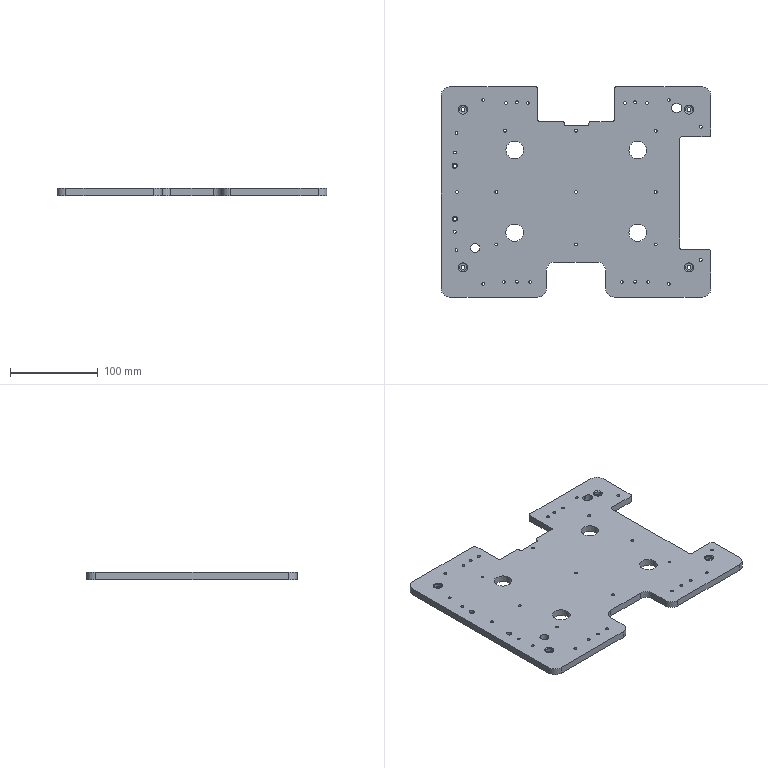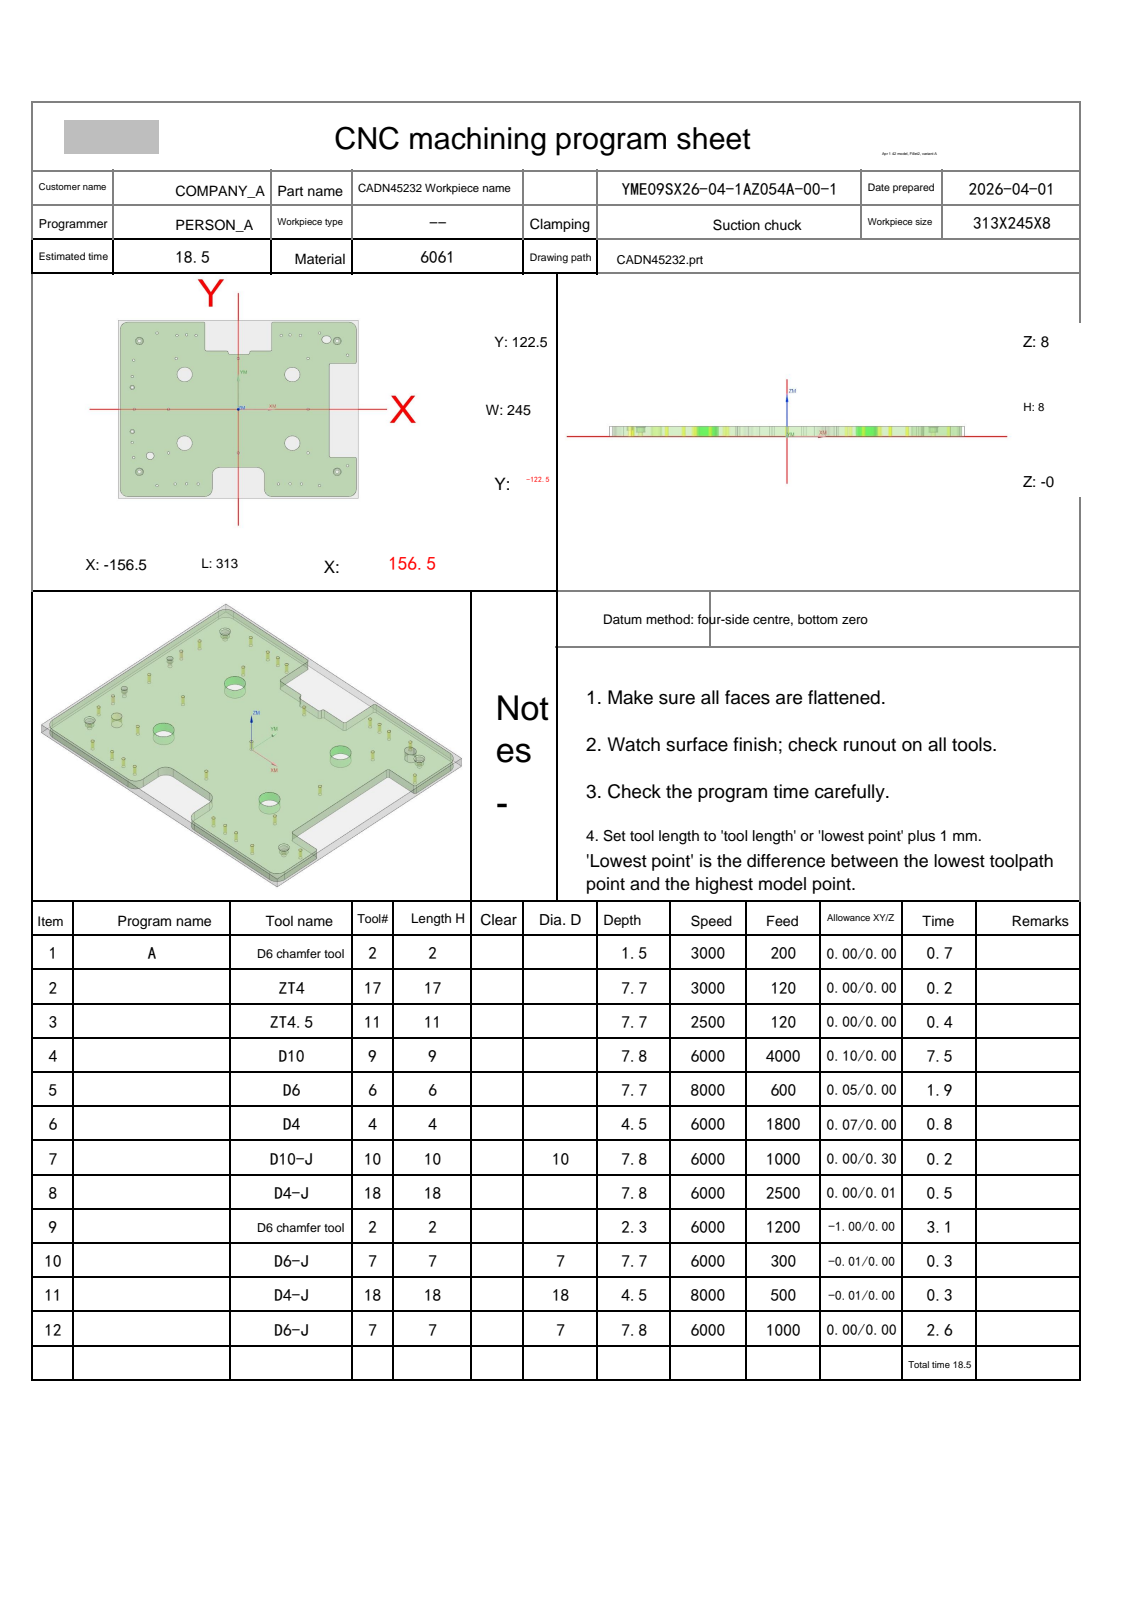NC program | NX | posted by the shop | part box 308 x 240 x 8 mm
Lines 1899 to 2964 of 6786:
N8 T18 M06
(D4-J  D=4. R=0. H=18 ce=0.00 di=0.01)
G00 G90 G54 X-40.899 Y85.842 M03 S6000
G43 H18 Z28.
M08
Z8.3
G01 X-40.906 Y85.841 Z8.214 F2000.
X-40.925 Y85.838 Z8.136
X-40.955 Y85.832 Z8.066
X-40.993 Y85.824 Z8.004
X-41.039 Y85.814 Z7.948
X-41.089 Y85.8 Z7.899
X-41.144 Y85.783 Z7.857
X-41.2 Y85.762 Z7.82
X-41.256 Y85.737 Z7.789
X-41.31 Y85.709 Z7.763
X-41.361 Y85.676 Z7.742
X-41.406 Y85.639 Z7.726
X-41.445 Y85.598 Z7.714
X-41.474 Y85.551 Z7.706
X-41.493 Y85.499 Z7.701
X-41.5 Y85.442 Z7.7
Y82.291 F2500.
X-41.459 Y82.289
X-41.387 Y82.303 Z7.699
X-41.308 Y82.349 Z7.695
X-41.224 Y82.423 Z7.689
X-41.138 Y82.521 Z7.681
X-41.053 Y82.641 Z7.671
X-40.972 Y82.779 Z7.659
X-40.897 Y82.932 Z7.647
X-40.832 Y83.096 Z7.633
X-40.78 Y83.268 Z7.619
X-40.729 Y83.535 Z7.596
X-40.711 Y83.806 Z7.573
X-40.724 Y84.078 Z7.55
X-40.767 Y84.344 Z7.527
X-40.836 Y84.6 Z7.504
X-40.931 Y84.84 Z7.481
X-40.999 Y84.975 Z7.468
X-41.072 Y85.1 Z7.456
X-41.148 Y85.212 Z7.444
X-41.224 Y85.309 Z7.434
X-41.296 Y85.39 Z7.424
X-41.361 Y85.45 Z7.416
X-41.418 Y85.488 Z7.409
X-41.461 Y85.5 Z7.404
X-41.49 Y85.486 Z7.401
X-41.5 Y85.442 Z7.4
Y82.291
X-41.459 Y82.289
X-41.387 Y82.303 Z7.399
X-41.308 Y82.349 Z7.395
X-41.224 Y82.422 Z7.39
X-41.138 Y82.521 Z7.382
X-41.053 Y82.641 Z7.373
X-40.972 Y82.779 Z7.363
X-40.897 Y82.931 Z7.351
X-40.832 Y83.095 Z7.338
X-40.78 Y83.267 Z7.324
X-40.729 Y83.534 Z7.302
X-40.711 Y83.805 Z7.279
X-40.724 Y84.077 Z7.255
X-40.767 Y84.343 Z7.231
X-40.836 Y84.599 Z7.207
X-40.931 Y84.84 Z7.184
X-40.999 Y84.975 Z7.171
X-41.072 Y85.099 Z7.158
X-41.148 Y85.212 Z7.146
X-41.224 Y85.309 Z7.135
X-41.296 Y85.389 Z7.125
X-41.361 Y85.45 Z7.117
X-41.418 Y85.487 Z7.11
X-41.461 Y85.5 Z7.104
X-41.49 Y85.486 Z7.101
X-41.5 Y85.442 Z7.1
Y82.291
X-41.459 Y82.289
X-41.387 Y82.303 Z7.099
X-41.308 Y82.349 Z7.095
X-41.224 Y82.422 Z7.09
X-41.138 Y82.521 Z7.082
X-41.053 Y82.64 Z7.073
X-40.971 Y82.778 Z7.063
X-40.897 Y82.931 Z7.051
X-40.832 Y83.094 Z7.038
X-40.78 Y83.266 Z7.024
X-40.729 Y83.532 Z7.002
X-40.711 Y83.804 Z6.979
X-40.724 Y84.076 Z6.955
X-40.766 Y84.342 Z6.931
X-40.836 Y84.598 Z6.907
X-40.931 Y84.839 Z6.884
X-40.999 Y84.974 Z6.871
X-41.072 Y85.099 Z6.858
X-41.148 Y85.211 Z6.846
X-41.224 Y85.309 Z6.835
X-41.296 Y85.389 Z6.825
X-41.361 Y85.449 Z6.817
X-41.418 Y85.487 Z6.81
X-41.461 Y85.5 Z6.804
X-41.49 Y85.486 Z6.801
X-41.5 Y85.442 Z6.8
Y82.291
X-41.459 Y82.289
X-41.387 Y82.303 Z6.799
X-41.308 Y82.348 Z6.795
X-41.224 Y82.422 Z6.79
X-41.138 Y82.52 Z6.782
X-41.053 Y82.64 Z6.773
X-40.971 Y82.777 Z6.762
X-40.897 Y82.93 Z6.75
X-40.832 Y83.093 Z6.737
X-40.779 Y83.265 Z6.724
X-40.729 Y83.531 Z6.702
X-40.711 Y83.803 Z6.678
X-40.724 Y84.075 Z6.655
X-40.766 Y84.341 Z6.631
X-40.836 Y84.598 Z6.607
X-40.931 Y84.839 Z6.584
X-40.999 Y84.974 Z6.571
X-41.072 Y85.098 Z6.558
X-41.148 Y85.211 Z6.546
X-41.224 Y85.309 Z6.535
X-41.296 Y85.389 Z6.525
X-41.361 Y85.449 Z6.517
X-41.418 Y85.487 Z6.51
X-41.461 Y85.5 Z6.504
X-41.49 Y85.486 Z6.501
X-41.5 Y85.442 Z6.5
Y82.291
X-41.459 Y82.289
X-41.387 Y82.303 Z6.499
X-41.308 Y82.348 Z6.495
X-41.224 Y82.422 Z6.49
X-41.138 Y82.52 Z6.482
X-41.053 Y82.639 Z6.473
X-40.971 Y82.777 Z6.462
X-40.897 Y82.929 Z6.45
X-40.832 Y83.092 Z6.437
X-40.779 Y83.264 Z6.423
X-40.729 Y83.53 Z6.401
X-40.711 Y83.802 Z6.378
X-40.724 Y84.074 Z6.355
X-40.766 Y84.34 Z6.331
X-40.836 Y84.597 Z6.307
X-40.931 Y84.838 Z6.284
X-40.999 Y84.973 Z6.271
X-41.072 Y85.098 Z6.258
X-41.148 Y85.211 Z6.246
X-41.224 Y85.308 Z6.235
X-41.296 Y85.389 Z6.225
X-41.361 Y85.449 Z6.217
X-41.418 Y85.487 Z6.21
X-41.461 Y85.5 Z6.204
X-41.49 Y85.486 Z6.201
X-41.5 Y85.442 Z6.2
Y82.291
X-41.459 Y82.289
X-41.387 Y82.303 Z6.199
X-41.308 Y82.348 Z6.195
X-41.224 Y82.421 Z6.19
X-41.138 Y82.519 Z6.182
X-41.053 Y82.639 Z6.173
X-40.971 Y82.776 Z6.162
X-40.897 Y82.928 Z6.15
X-40.832 Y83.092 Z6.137
X-40.779 Y83.263 Z6.123
X-40.729 Y83.529 Z6.101
X-40.711 Y83.801 Z6.078
X-40.724 Y84.073 Z6.054
X-40.766 Y84.339 Z6.03
X-40.836 Y84.596 Z6.007
X-40.931 Y84.837 Z5.984
X-40.999 Y84.973 Z5.97
X-41.072 Y85.098 Z5.958
X-41.148 Y85.21 Z5.946
X-41.224 Y85.308 Z5.935
X-41.296 Y85.389 Z5.925
X-41.361 Y85.449 Z5.916
X-41.418 Y85.487 Z5.91
X-41.461 Y85.5 Z5.904
X-41.49 Y85.486 Z5.901
X-41.5 Y85.442 Z5.9
Y82.291
X-41.459 Y82.289
X-41.387 Y82.303 Z5.899
X-41.308 Y82.348 Z5.895
X-41.224 Y82.421 Z5.89
X-41.138 Y82.519 Z5.882
X-41.053 Y82.638 Z5.873
X-40.971 Y82.775 Z5.862
X-40.897 Y82.927 Z5.85
X-40.832 Y83.091 Z5.837
X-40.779 Y83.262 Z5.823
X-40.728 Y83.528 Z5.801
X-40.711 Y83.8 Z5.778
X-40.724 Y84.071 Z5.754
X-40.766 Y84.338 Z5.73
X-40.836 Y84.595 Z5.707
X-40.931 Y84.837 Z5.684
X-40.999 Y84.972 Z5.67
X-41.072 Y85.097 Z5.658
X-41.148 Y85.21 Z5.646
X-41.224 Y85.308 Z5.635
X-41.296 Y85.388 Z5.625
X-41.361 Y85.449 Z5.616
X-41.418 Y85.487 Z5.61
X-41.461 Y85.5 Z5.604
X-41.49 Y85.486 Z5.601
X-41.5 Y85.442 Z5.6
Y82.291
X-41.422 Y82.289
X-41.351 Y82.304 Z5.599
X-41.272 Y82.351 Z5.595
X-41.188 Y82.426 Z5.59
X-41.103 Y82.525 Z5.582
X-41.019 Y82.646 Z5.573
X-40.94 Y82.784 Z5.562
X-40.867 Y82.937 Z5.55
X-40.803 Y83.101 Z5.537
X-40.753 Y83.273 Z5.523
X-40.705 Y83.54 Z5.501
X-40.69 Y83.811 Z5.478
X-40.706 Y84.082 Z5.455
X-40.751 Y84.347 Z5.431
X-40.823 Y84.603 Z5.407
X-40.921 Y84.843 Z5.384
X-40.991 Y84.977 Z5.371
X-41.065 Y85.101 Z5.358
X-41.143 Y85.213 Z5.346
X-41.22 Y85.31 Z5.335
X-41.293 Y85.39 Z5.325
X-41.359 Y85.45 Z5.317
X-41.416 Y85.488 Z5.31
X-41.461 Y85.501 Z5.304
X-41.49 Y85.486 Z5.301
X-41.5 Y85.442 Z5.3
Y82.291
X-41.422 Y82.289
X-41.351 Y82.304 Z5.299
X-41.272 Y82.351 Z5.295
X-41.188 Y82.425 Z5.29
X-41.103 Y82.524 Z5.282
X-41.019 Y82.645 Z5.273
X-40.939 Y82.783 Z5.262
X-40.866 Y82.936 Z5.25
X-40.803 Y83.1 Z5.237
X-40.753 Y83.272 Z5.223
X-40.705 Y83.538 Z5.201
X-40.69 Y83.809 Z5.178
X-40.706 Y84.08 Z5.154
X-40.751 Y84.346 Z5.13
X-40.823 Y84.602 Z5.107
X-40.921 Y84.842 Z5.084
X-40.99 Y84.976 Z5.07
X-41.065 Y85.101 Z5.058
X-41.143 Y85.213 Z5.046
X-41.22 Y85.31 Z5.035
X-41.293 Y85.39 Z5.025
X-41.359 Y85.45 Z5.016
X-41.416 Y85.488 Z5.01
X-41.461 Y85.501 Z5.004
X-41.49 Y85.486 Z5.001
X-41.5 Y85.442 Z5.
Y82.291
X-41.422 Y82.289
X-41.351 Y82.304 Z4.999
X-41.272 Y82.351 Z4.995
X-41.188 Y82.425 Z4.99
X-41.103 Y82.524 Z4.982
X-41.019 Y82.644 Z4.973
X-40.939 Y82.782 Z4.962
X-40.866 Y82.935 Z4.95
X-40.803 Y83.099 Z4.937
X-40.752 Y83.27 Z4.923
X-40.704 Y83.536 Z4.901
X-40.689 Y83.808 Z4.878
X-40.706 Y84.079 Z4.854
X-40.751 Y84.345 Z4.83
X-40.823 Y84.601 Z4.807
X-40.921 Y84.841 Z4.784
X-40.99 Y84.976 Z4.77
X-41.065 Y85.1 Z4.758
X-41.143 Y85.212 Z4.746
X-41.22 Y85.31 Z4.735
X-41.293 Y85.39 Z4.725
X-41.359 Y85.45 Z4.716
X-41.416 Y85.488 Z4.71
X-41.461 Y85.501 Z4.704
X-41.49 Y85.486 Z4.701
X-41.5 Y85.442 Z4.7
Y82.291
X-41.422 Y82.289
X-41.351 Y82.304 Z4.699
X-41.272 Y82.351 Z4.695
X-41.188 Y82.426 Z4.689
X-41.103 Y82.525 Z4.681
X-41.019 Y82.646 Z4.671
X-40.94 Y82.784 Z4.659
X-40.866 Y82.937 Z4.647
X-40.803 Y83.101 Z4.633
X-40.753 Y83.273 Z4.619
X-40.705 Y83.54 Z4.596
X-40.69 Y83.811 Z4.573
X-40.706 Y84.082 Z4.55
X-40.751 Y84.347 Z4.527
X-40.823 Y84.603 Z4.504
X-40.921 Y84.843 Z4.481
X-40.991 Y84.977 Z4.468
X-41.065 Y85.101 Z4.456
X-41.143 Y85.213 Z4.444
X-41.22 Y85.31 Z4.434
X-41.293 Y85.39 Z4.424
X-41.359 Y85.45 Z4.416
X-41.416 Y85.488 Z4.409
X-41.461 Y85.501 Z4.404
X-41.49 Y85.486 Z4.401
X-41.5 Y85.442 Z4.4
Y82.291
X-41.422 Y82.289
X-41.351 Y82.304 Z4.399
X-41.272 Y82.351 Z4.395
X-41.188 Y82.425 Z4.389
X-41.103 Y82.524 Z4.381
X-41.019 Y82.645 Z4.371
X-40.939 Y82.783 Z4.359
X-40.866 Y82.936 Z4.347
X-40.803 Y83.1 Z4.333
X-40.752 Y83.272 Z4.319
X-40.704 Y83.538 Z4.296
X-40.69 Y83.809 Z4.273
X-40.706 Y84.08 Z4.25
X-40.751 Y84.346 Z4.227
X-40.823 Y84.602 Z4.204
X-40.921 Y84.842 Z4.181
X-40.99 Y84.976 Z4.168
X-41.065 Y85.101 Z4.156
X-41.143 Y85.213 Z4.144
X-41.22 Y85.31 Z4.134
X-41.293 Y85.39 Z4.124
X-41.359 Y85.45 Z4.116
X-41.416 Y85.488 Z4.109
X-41.461 Y85.501 Z4.104
X-41.49 Y85.486 Z4.101
X-41.5 Y85.442 Z4.1
Y82.291
X-41.422 Y82.289
X-41.351 Y82.304 Z4.099
X-41.272 Y82.351 Z4.095
X-41.188 Y82.425 Z4.09
X-41.103 Y82.524 Z4.083
X-41.019 Y82.644 Z4.074
X-40.939 Y82.782 Z4.063
X-40.866 Y82.934 Z4.052
X-40.803 Y83.098 Z4.039
X-40.752 Y83.27 Z4.025
X-40.704 Y83.536 Z4.003
X-40.689 Y83.807 Z3.98
X-40.706 Y84.078 Z3.956
X-40.751 Y84.344 Z3.932
X-40.823 Y84.6 Z3.908
X-40.921 Y84.841 Z3.885
X-40.99 Y84.975 Z3.871
X-41.065 Y85.1 Z3.859
X-41.143 Y85.212 Z3.846
X-41.22 Y85.31 Z3.835
X-41.293 Y85.39 Z3.825
X-41.359 Y85.45 Z3.817
X-41.416 Y85.488 Z3.81
X-41.461 Y85.501 Z3.804
X-41.49 Y85.486 Z3.801
X-41.5 Y85.442 Z3.8
Y82.291
X-41.422 Y82.289
X-41.351 Y82.304 Z3.799
X-41.272 Y82.35 Z3.795
X-41.188 Y82.425 Z3.79
X-41.103 Y82.523 Z3.783
X-41.019 Y82.643 Z3.774
X-40.939 Y82.781 Z3.763
X-40.866 Y82.933 Z3.751
X-40.803 Y83.097 Z3.739
X-40.752 Y83.268 Z3.725
X-40.704 Y83.534 Z3.703
X-40.689 Y83.805 Z3.68
X-40.705 Y84.077 Z3.656
X-40.751 Y84.343 Z3.632
X-40.823 Y84.599 Z3.608
X-40.921 Y84.84 Z3.585
X-40.99 Y84.974 Z3.571
X-41.065 Y85.099 Z3.558
X-41.143 Y85.212 Z3.546
X-41.219 Y85.309 Z3.535
X-41.293 Y85.389 Z3.525
X-41.359 Y85.45 Z3.517
X-41.416 Y85.487 Z3.51
X-41.461 Y85.5 Z3.504
X-41.49 Y85.486 Z3.501
X-41.5 Y85.442 Z3.5
Y82.291
X-41.422 Y82.289
X-41.351 Y82.304 Z3.499
X-41.272 Y82.35 Z3.495
X-41.188 Y82.424 Z3.49
X-41.103 Y82.523 Z3.482
X-41.019 Y82.642 Z3.473
X-40.939 Y82.78 Z3.463
X-40.866 Y82.932 Z3.451
X-40.803 Y83.095 Z3.438
X-40.752 Y83.266 Z3.424
X-40.704 Y83.532 Z3.402
X-40.689 Y83.803 Z3.379
X-40.705 Y84.075 Z3.355
X-40.75 Y84.341 Z3.331
X-40.823 Y84.598 Z3.308
X-40.921 Y84.839 Z3.284
X-40.99 Y84.974 Z3.271
X-41.065 Y85.099 Z3.258
X-41.143 Y85.211 Z3.246
X-41.219 Y85.309 Z3.235
X-41.293 Y85.389 Z3.225
X-41.359 Y85.449 Z3.217
X-41.416 Y85.487 Z3.21
X-41.461 Y85.5 Z3.204
X-41.49 Y85.486 Z3.201
X-41.5 Y85.442 Z3.2
Y82.291
X-41.422 Y82.289
X-41.35 Y82.304 Z3.199
X-41.272 Y82.35 Z3.195
X-41.188 Y82.424 Z3.19
X-41.103 Y82.522 Z3.182
X-41.019 Y82.641 Z3.173
X-40.939 Y82.778 Z3.163
X-40.866 Y82.93 Z3.151
X-40.803 Y83.093 Z3.138
X-40.752 Y83.265 Z3.124
X-40.704 Y83.53 Z3.102
X-40.689 Y83.802 Z3.079
X-40.705 Y84.073 Z3.055
X-40.75 Y84.34 Z3.031
X-40.823 Y84.597 Z3.007
X-40.921 Y84.838 Z2.984
X-40.99 Y84.973 Z2.971
X-41.065 Y85.098 Z2.958
X-41.143 Y85.211 Z2.946
X-41.219 Y85.308 Z2.935
X-41.293 Y85.389 Z2.925
X-41.359 Y85.449 Z2.917
X-41.416 Y85.487 Z2.91
X-41.461 Y85.5 Z2.904
X-41.49 Y85.486 Z2.901
X-41.5 Y85.442 Z2.9
Y82.291
X-41.422 Y82.289
X-41.35 Y82.304 Z2.899
X-41.272 Y82.35 Z2.895
X-41.188 Y82.423 Z2.89
X-41.103 Y82.521 Z2.882
X-41.019 Y82.64 Z2.873
X-40.939 Y82.777 Z2.862
X-40.866 Y82.929 Z2.85
X-40.802 Y83.092 Z2.837
X-40.752 Y83.263 Z2.823
X-40.704 Y83.528 Z2.801
X-40.689 Y83.8 Z2.778
X-40.705 Y84.071 Z2.754
X-40.75 Y84.338 Z2.731
X-40.823 Y84.595 Z2.707
X-40.921 Y84.837 Z2.684
X-40.99 Y84.972 Z2.671
X-41.065 Y85.097 Z2.658
X-41.143 Y85.21 Z2.646
X-41.219 Y85.308 Z2.635
X-41.293 Y85.388 Z2.625
X-41.359 Y85.449 Z2.617
X-41.416 Y85.487 Z2.61
X-41.461 Y85.5 Z2.604
X-41.49 Y85.486 Z2.601
X-41.5 Y85.442 Z2.6
Y82.291
X-41.422 Y82.289
X-41.341 Y82.308 Z2.598
X-41.251 Y82.366 Z2.594
X-41.156 Y82.457 Z2.587
X-41.061 Y82.578 Z2.578
X-40.968 Y82.723 Z2.566
X-40.883 Y82.888 Z2.553
X-40.81 Y83.069 Z2.538
X-40.752 Y83.261 Z2.523
X-40.704 Y83.527 Z2.501
X-40.689 Y83.798 Z2.478
X-40.705 Y84.07 Z2.454
X-40.75 Y84.337 Z2.43
X-40.823 Y84.594 Z2.407
X-40.92 Y84.836 Z2.384
X-40.99 Y84.971 Z2.37
X-41.065 Y85.097 Z2.358
X-41.143 Y85.209 Z2.346
X-41.219 Y85.308 Z2.335
X-41.293 Y85.388 Z2.325
X-41.359 Y85.449 Z2.316
X-41.416 Y85.487 Z2.31
X-41.461 Y85.5 Z2.304
X-41.49 Y85.486 Z2.301
X-41.5 Y85.442 Z2.3
Y82.291
X-41.422 Y82.289
X-41.341 Y82.308 Z2.298
X-41.251 Y82.365 Z2.294
X-41.156 Y82.457 Z2.287
X-41.061 Y82.577 Z2.277
X-40.968 Y82.722 Z2.266
X-40.883 Y82.887 Z2.253
X-40.81 Y83.068 Z2.238
X-40.752 Y83.259 Z2.222
X-40.704 Y83.525 Z2.2
X-40.689 Y83.796 Z2.177
X-40.705 Y84.068 Z2.154
X-40.75 Y84.335 Z2.13
X-40.823 Y84.593 Z2.106
X-40.92 Y84.835 Z2.083
X-40.99 Y84.97 Z2.07
X-41.065 Y85.096 Z2.057
X-41.143 Y85.209 Z2.046
X-41.219 Y85.307 Z2.035
X-41.293 Y85.388 Z2.025
X-41.359 Y85.449 Z2.016
X-41.416 Y85.487 Z2.01
X-41.461 Y85.5 Z2.004
X-41.49 Y85.486 Z2.001
X-41.5 Y85.442 Z2.
Y82.291
X-41.422 Y82.289
X-41.341 Y82.308 Z1.998
X-41.251 Y82.365 Z1.994
X-41.156 Y82.456 Z1.987
X-41.061 Y82.576 Z1.977
X-40.968 Y82.721 Z1.966
X-40.883 Y82.886 Z1.952
X-40.809 Y83.066 Z1.938
X-40.751 Y83.258 Z1.922
X-40.703 Y83.523 Z1.9
X-40.689 Y83.794 Z1.877
X-40.705 Y84.066 Z1.853
X-40.75 Y84.334 Z1.829
X-40.823 Y84.591 Z1.806
X-40.92 Y84.834 Z1.783
X-40.99 Y84.969 Z1.77
X-41.065 Y85.095 Z1.757
X-41.142 Y85.208 Z1.745
X-41.219 Y85.307 Z1.734
X-41.293 Y85.388 Z1.725
X-41.359 Y85.448 Z1.716
X-41.416 Y85.487 Z1.709
X-41.461 Y85.5 Z1.704
X-41.49 Y85.486 Z1.701
X-41.5 Y85.442 Z1.7
Y82.291
X-41.422 Y82.289
X-41.341 Y82.308 Z1.698
X-41.251 Y82.365 Z1.694
X-41.156 Y82.456 Z1.687
X-41.06 Y82.576 Z1.677
X-40.968 Y82.72 Z1.665
X-40.883 Y82.885 Z1.652
X-40.809 Y83.065 Z1.637
X-40.751 Y83.256 Z1.621
X-40.703 Y83.521 Z1.599
X-40.688 Y83.792 Z1.576
X-40.705 Y84.065 Z1.553
X-40.75 Y84.332 Z1.529
X-40.822 Y84.59 Z1.506
X-40.92 Y84.833 Z1.483
X-40.99 Y84.969 Z1.47
X-41.065 Y85.094 Z1.457
X-41.142 Y85.208 Z1.445
X-41.219 Y85.306 Z1.434
X-41.293 Y85.387 Z1.425
X-41.359 Y85.448 Z1.416
X-41.416 Y85.487 Z1.409
X-41.461 Y85.5 Z1.404
X-41.49 Y85.486 Z1.401
X-41.5 Y85.442 Z1.4
Y82.291
X-41.422 Y82.289
X-41.341 Y82.308 Z1.398
X-41.251 Y82.365 Z1.394
X-41.156 Y82.455 Z1.386
X-41.06 Y82.575 Z1.377
X-40.968 Y82.719 Z1.365
X-40.883 Y82.883 Z1.352
X-40.809 Y83.063 Z1.337
X-40.751 Y83.254 Z1.321
X-40.703 Y83.519 Z1.299
X-40.688 Y83.79 Z1.276
X-40.705 Y84.063 Z1.252
X-40.75 Y84.331 Z1.229
X-40.822 Y84.589 Z1.205
X-40.92 Y84.832 Z1.182
X-40.99 Y84.968 Z1.169
X-41.065 Y85.094 Z1.157
X-41.142 Y85.207 Z1.145
X-41.219 Y85.306 Z1.134
X-41.293 Y85.387 Z1.125
X-41.359 Y85.448 Z1.116
X-41.416 Y85.487 Z1.109
X-41.461 Y85.5 Z1.104
X-41.49 Y85.486 Z1.101
X-41.5 Y85.442 Z1.1
Y82.291
X-41.422 Y82.289
X-41.341 Y82.308 Z1.098
X-41.251 Y82.364 Z1.094
X-41.156 Y82.455 Z1.086
X-41.06 Y82.574 Z1.077
X-40.968 Y82.718 Z1.065
X-40.883 Y82.882 Z1.051
X-40.809 Y83.061 Z1.036
X-40.751 Y83.252 Z1.02
X-40.703 Y83.517 Z.998
X-40.688 Y83.789 Z.975
X-40.704 Y84.061 Z.952
X-40.75 Y84.329 Z.928
X-40.822 Y84.588 Z.905
X-40.92 Y84.831 Z.882
X-40.99 Y84.967 Z.869
X-41.065 Y85.093 Z.857
X-41.142 Y85.207 Z.845
X-41.219 Y85.305 Z.834
X-41.293 Y85.387 Z.825
X-41.359 Y85.448 Z.816
X-41.416 Y85.486 Z.809
X-41.461 Y85.5 Z.804
X-41.49 Y85.486 Z.801
X-41.5 Y85.442 Z.8
Y82.291
X-41.422 Y82.289
X-41.341 Y82.308 Z.798
X-41.251 Y82.364 Z.794
X-41.156 Y82.454 Z.786
X-41.06 Y82.573 Z.776
X-40.968 Y82.717 Z.764
X-40.883 Y82.881 Z.751
X-40.809 Y83.06 Z.736
X-40.751 Y83.251 Z.72
X-40.703 Y83.515 Z.698
X-40.688 Y83.787 Z.675
X-40.704 Y84.059 Z.651
X-40.75 Y84.328 Z.628
X-40.822 Y84.586 Z.604
X-40.92 Y84.83 Z.582
X-40.99 Y84.966 Z.569
X-41.065 Y85.092 Z.556
X-41.142 Y85.206 Z.545
X-41.219 Y85.305 Z.534
X-41.293 Y85.386 Z.524
X-41.359 Y85.448 Z.516
X-41.416 Y85.486 Z.509
X-41.461 Y85.5 Z.504
X-41.49 Y85.486 Z.501
X-41.5 Y85.442 Z.5
Y82.291
X-41.422 Y82.289
X-41.341 Y82.308 Z.498
X-41.251 Y82.364 Z.494
X-41.156 Y82.454 Z.486
X-41.06 Y82.573 Z.476
X-40.968 Y82.716 Z.464
X-40.883 Y82.879 Z.45
X-40.809 Y83.058 Z.435
X-40.751 Y83.249 Z.42
X-40.703 Y83.513 Z.397
X-40.688 Y83.785 Z.374
X-40.704 Y84.058 Z.351
X-40.75 Y84.326 Z.327
X-40.822 Y84.585 Z.304
X-40.92 Y84.829 Z.282
X-40.99 Y84.965 Z.269
X-41.065 Y85.092 Z.256
X-41.142 Y85.206 Z.245
X-41.219 Y85.305 Z.234
X-41.293 Y85.386 Z.224
X-41.359 Y85.447 Z.216
X-41.416 Y85.486 Z.209
X-41.461 Y85.5 Z.204
X-41.49 Y85.486 Z.201
X-41.5 Y85.442 Z.2
Y82.291
X-41.422 Y82.289
Z.8
G00 Z28.
X-10.73 Y79.374
Z8.3
G01 X-10.738 Y79.371 Z8.209 F2000.
X-10.758 Y79.362 Z8.127
X-10.789 Y79.347 Z8.053
X-10.829 Y79.327 Z7.988
X-10.876 Y79.301 Z7.931
X-10.928 Y79.271 Z7.881
X-10.982 Y79.236 Z7.839
X-11.036 Y79.196 Z7.803
X-11.089 Y79.153 Z7.773
X-11.138 Y79.105 Z7.749
X-11.182 Y79.054 Z7.73
X-11.217 Y79. Z7.716
X-11.242 Y78.943 Z7.707
X-11.256 Y78.883 Z7.702
X-11.255 Y78.821 Z7.7
G02 X-11.216 Y78.281 I-4.026 J-.558 F2500.
G01 Y77.706
X-8.496
X-8.449 Y77.718 Z7.699
X-8.425 Y77.753 Z7.696
X-8.424 Y77.808 Z7.691
X-8.442 Y77.878 Z7.684
X-8.478 Y77.961 Z7.676
X-8.53 Y78.053 Z7.666
X-8.596 Y78.151 Z7.656
X-8.675 Y78.251 Z7.644
X-8.763 Y78.351 Z7.632
X-8.86 Y78.446 Z7.619
X-9.073 Y78.614 Z7.592
X-9.31 Y78.753 Z7.564
X-9.57 Y78.862 Z7.536
X-9.852 Y78.943 Z7.508
X-10.155 Y78.997 Z7.481
X-10.314 Y79.014 Z7.468
X-10.473 Y79.023 Z7.456
X-10.628 Y79.026 Z7.444
X-10.776 Y79.021 Z7.434
X-10.911 Y79.008 Z7.424
X-11.03 Y78.988 Z7.416
X-11.128 Y78.959 Z7.409
X-11.201 Y78.922 Z7.404
X-11.245 Y78.876 Z7.401
X-11.255 Y78.821 Z7.4
G02 X-11.216 Y78.281 I-4.026 J-.558
G01 Y77.706
X-8.496
X-8.449 Y77.718 Z7.399
X-8.425 Y77.753 Z7.396
X-8.424 Y77.808 Z7.391
X-8.442 Y77.878 Z7.385
X-8.478 Y77.961 Z7.377
X-8.53 Y78.053 Z7.367
X-8.596 Y78.151 Z7.357
X-8.675 Y78.252 Z7.346
X-8.763 Y78.351 Z7.334
X-8.86 Y78.446 Z7.322
X-9.073 Y78.615 Z7.296
X-9.31 Y78.754 Z7.269
X-9.57 Y78.863 Z7.241
X-9.853 Y78.945 Z7.214
X-10.156 Y78.998 Z7.187
X-10.314 Y79.015 Z7.173
X-10.473 Y79.024 Z7.16
X-10.628 Y79.027 Z7.148
X-10.776 Y79.022 Z7.137
X-10.911 Y79.009 Z7.126
X-11.03 Y78.988 Z7.118
X-11.128 Y78.959 Z7.11
X-11.201 Y78.922 Z7.105
X-11.245 Y78.876 Z7.101
X-11.255 Y78.821 Z7.1
G02 X-11.216 Y78.281 I-4.026 J-.558
G01 Y77.706
X-8.496
X-8.449 Y77.718 Z7.099
X-8.425 Y77.753 Z7.096
X-8.424 Y77.808 Z7.091
X-8.442 Y77.878 Z7.085
X-8.478 Y77.961 Z7.077
X-8.53 Y78.053 Z7.067
X-8.596 Y78.151 Z7.057
X-8.675 Y78.252 Z7.046
X-8.763 Y78.352 Z7.034
X-8.86 Y78.447 Z7.022
X-9.073 Y78.616 Z6.996
X-9.311 Y78.755 Z6.969
X-9.571 Y78.864 Z6.941
X-9.853 Y78.946 Z6.914
X-10.156 Y78.999 Z6.886
X-10.314 Y79.016 Z6.873
X-10.473 Y79.025 Z6.86
X-10.629 Y79.027 Z6.848
X-10.776 Y79.022 Z6.837
X-10.911 Y79.009 Z6.826
X-11.03 Y78.989 Z6.817
X-11.128 Y78.959 Z6.81
X-11.201 Y78.922 Z6.805
X-11.245 Y78.876 Z6.801
X-11.255 Y78.821 Z6.8
G02 X-11.216 Y78.281 I-4.026 J-.558
G01 Y77.706
X-8.496
X-8.449 Y77.718 Z6.799
X-8.425 Y77.753 Z6.796
X-8.424 Y77.808 Z6.791
X-8.442 Y77.878 Z6.785
X-8.478 Y77.961 Z6.777
X-8.53 Y78.054 Z6.767
X-8.597 Y78.152 Z6.757
X-8.675 Y78.252 Z6.746
X-8.764 Y78.352 Z6.734
X-8.86 Y78.447 Z6.721
X-9.074 Y78.616 Z6.695
X-9.311 Y78.756 Z6.668
X-9.571 Y78.866 Z6.641
X-9.853 Y78.947 Z6.613
X-10.156 Y79. Z6.586
X-10.314 Y79.017 Z6.573
X-10.473 Y79.026 Z6.56
X-10.629 Y79.028 Z6.548
X-10.776 Y79.023 Z6.536
X-10.911 Y79.01 Z6.526
X-11.03 Y78.989 Z6.517
X-11.128 Y78.96 Z6.51
X-11.201 Y78.922 Z6.505
X-11.245 Y78.876 Z6.501
X-11.255 Y78.821 Z6.5
G02 X-11.216 Y78.281 I-4.026 J-.558
G01 Y77.706
X-8.496
X-8.449 Y77.718 Z6.499
X-8.425 Y77.753 Z6.496
X-8.424 Y77.808 Z6.491
X-8.442 Y77.878 Z6.485
X-8.478 Y77.962 Z6.477
X-8.53 Y78.054 Z6.467
X-8.597 Y78.152 Z6.457
X-8.675 Y78.253 Z6.446
X-8.764 Y78.353 Z6.434
X-8.861 Y78.448 Z6.421
X-9.074 Y78.617 Z6.395
X-9.311 Y78.757 Z6.368
X-9.571 Y78.867 Z6.341
X-9.853 Y78.948 Z6.313
X-10.156 Y79.001 Z6.286
X-10.315 Y79.018 Z6.273
X-10.474 Y79.027 Z6.26
X-10.629 Y79.029 Z6.248
X-10.776 Y79.023 Z6.236
X-10.912 Y79.01 Z6.226
X-11.03 Y78.989 Z6.217
X-11.128 Y78.96 Z6.21
X-11.201 Y78.922 Z6.205
X-11.245 Y78.876 Z6.201
X-11.255 Y78.821 Z6.2
G02 X-11.216 Y78.281 I-4.026 J-.557
G01 Y77.706
X-8.496
X-8.449 Y77.718 Z6.199
X-8.425 Y77.753 Z6.196
X-8.424 Y77.808 Z6.191
X-8.442 Y77.879 Z6.184
X-8.478 Y77.962 Z6.177
X-8.53 Y78.054 Z6.167
X-8.597 Y78.152 Z6.157
X-8.675 Y78.253 Z6.146
X-8.764 Y78.353 Z6.134
X-8.861 Y78.449 Z6.121
X-9.074 Y78.618 Z6.095
X-9.311 Y78.758 Z6.068
X-9.572 Y78.868 Z6.04
X-9.854 Y78.949 Z6.013
X-10.157 Y79.002 Z5.986
X-10.315 Y79.019 Z5.972
X-10.474 Y79.028 Z5.96
X-10.629 Y79.03 Z5.947
X-10.776 Y79.024 Z5.936
X-10.912 Y79.011 Z5.926
X-11.03 Y78.989 Z5.917
X-11.128 Y78.96 Z5.91
X-11.201 Y78.922 Z5.905
X-11.245 Y78.876 Z5.901
X-11.255 Y78.821 Z5.9
G02 X-11.216 Y78.281 I-4.026 J-.557
G01 Y77.706
X-8.496
X-8.449 Y77.718 Z5.899
X-8.425 Y77.753 Z5.896
X-8.424 Y77.808 Z5.891
X-8.442 Y77.879 Z5.884
X-8.478 Y77.962 Z5.876
X-8.53 Y78.054 Z5.867
X-8.597 Y78.153 Z5.857
X-8.675 Y78.254 Z5.846
X-8.764 Y78.354 Z5.834
X-8.861 Y78.449 Z5.821
X-9.074 Y78.619 Z5.795
X-9.312 Y78.758 Z5.768
X-9.572 Y78.869 Z5.74
X-9.854 Y78.95 Z5.713
X-10.157 Y79.003 Z5.685
X-10.315 Y79.02 Z5.672
X-10.474 Y79.029 Z5.659
X-10.629 Y79.03 Z5.647
X-10.777 Y79.025 Z5.636
X-10.912 Y79.011 Z5.626
X-11.03 Y78.99 Z5.617
X-11.128 Y78.96 Z5.61
X-11.201 Y78.922 Z5.605
X-11.245 Y78.876 Z5.601
X-11.255 Y78.821 Z5.6
G02 X-11.216 Y78.281 I-4.026 J-.557
G01 Y77.706
X-8.496
X-8.449 Y77.718 Z5.599
X-8.425 Y77.753 Z5.596
X-8.424 Y77.808 Z5.591
X-8.442 Y77.879 Z5.584
X-8.478 Y77.962 Z5.576
X-8.53 Y78.055 Z5.567
X-8.597 Y78.153 Z5.557
X-8.675 Y78.254 Z5.546
X-8.764 Y78.354 Z5.534
X-8.861 Y78.45 Z5.521
X-9.074 Y78.62 Z5.495
X-9.312 Y78.759 Z5.468
X-9.572 Y78.87 Z5.44
X-9.854 Y78.951 Z5.412
X-10.157 Y79.004 Z5.385
X-10.316 Y79.021 Z5.372
X-10.474 Y79.029 Z5.359
X-10.63 Y79.031 Z5.347
X-10.777 Y79.025 Z5.336
X-10.912 Y79.012 Z5.326
X-11.03 Y78.99 Z5.317
X-11.128 Y78.96 Z5.31
X-11.201 Y78.923 Z5.305
X-11.245 Y78.876 Z5.301
X-11.255 Y78.821 Z5.3
G02 X-11.216 Y78.281 I-4.026 J-.557
G01 Y77.706
X-8.496
X-8.449 Y77.718 Z5.299
X-8.425 Y77.753 Z5.296
X-8.424 Y77.808 Z5.291
X-8.442 Y77.879 Z5.284
X-8.478 Y77.962 Z5.276
X-8.531 Y78.055 Z5.267
X-8.597 Y78.153 Z5.257
X-8.676 Y78.254 Z5.245
X-8.764 Y78.354 Z5.233
X-8.861 Y78.45 Z5.221
X-9.075 Y78.62 Z5.195
X-9.312 Y78.76 Z5.167
X-9.573 Y78.871 Z5.14
X-9.855 Y78.952 Z5.112
X-10.158 Y79.005 Z5.085
X-10.316 Y79.021 Z5.072
X-10.475 Y79.03 Z5.059
X-10.63 Y79.032 Z5.047
X-10.777 Y79.026 Z5.036
X-10.912 Y79.012 Z5.026
X-11.031 Y78.99 Z5.017
X-11.128 Y78.961 Z5.01
X-11.201 Y78.923 Z5.005
X-11.245 Y78.876 Z5.001
X-11.255 Y78.821 Z5.
G02 X-11.216 Y78.281 I-4.026 J-.557
G01 Y77.706
X-8.496
X-8.449 Y77.718 Z4.999
X-8.425 Y77.753 Z4.996
X-8.424 Y77.808 Z4.991
X-8.442 Y77.879 Z4.984
X-8.478 Y77.962 Z4.976
X-8.531 Y78.055 Z4.967
X-8.597 Y78.154 Z4.957
X-8.676 Y78.255 Z4.945
X-8.764 Y78.355 Z4.933
X-8.862 Y78.451 Z4.921
X-9.075 Y78.621 Z4.894
X-9.312 Y78.761 Z4.867
X-9.573 Y78.872 Z4.84
X-9.855 Y78.954 Z4.812
X-10.158 Y79.007 Z4.785
X-10.316 Y79.022 Z4.772
X-10.475 Y79.031 Z4.759
X-10.63 Y79.032 Z4.747
X-10.777 Y79.026 Z4.736
X-10.912 Y79.012 Z4.726
X-11.031 Y78.991 Z4.717
X-11.128 Y78.961 Z4.71
X-11.201 Y78.923 Z4.705
X-11.245 Y78.876 Z4.701
X-11.255 Y78.821 Z4.7
G02 X-11.216 Y78.281 I-4.023 J-.557
G01 Y77.706
X-8.496
X-8.449 Y77.718 Z4.699
X-8.425 Y77.754 Z4.696
X-8.424 Y77.808 Z4.691
X-8.442 Y77.879 Z4.684
X-8.478 Y77.963 Z4.676
X-8.531 Y78.055 Z4.667
X-8.597 Y78.154 Z4.657
X-8.676 Y78.255 Z4.645
X-8.765 Y78.355 Z4.633
X-8.862 Y78.452 Z4.621
X-9.075 Y78.622 Z4.594
X-9.313 Y78.762 Z4.567
X-9.573 Y78.873 Z4.539
X-9.856 Y78.955 Z4.512
X-10.158 Y79.008 Z4.485
X-10.316 Y79.023 Z4.471
X-10.475 Y79.032 Z4.459
X-10.63 Y79.033 Z4.447
X-10.777 Y79.027 Z4.436
X-10.912 Y79.013 Z4.426
X-11.031 Y78.991 Z4.417
X-11.128 Y78.961 Z4.41
X-11.201 Y78.923 Z4.405
X-11.245 Y78.876 Z4.401
X-11.255 Y78.821 Z4.4
G02 X-11.216 Y78.283 I-4.009 J-.556
G01 Y77.706
X-8.496
X-8.449 Y77.718 Z4.399
X-8.425 Y77.754 Z4.396
X-8.424 Y77.808 Z4.391
X-8.442 Y77.879 Z4.384
X-8.478 Y77.963 Z4.376
X-8.531 Y78.056 Z4.367
X-8.597 Y78.154 Z4.357
X-8.676 Y78.256 Z4.345
X-8.765 Y78.356 Z4.333
X-8.862 Y78.452 Z4.32
X-9.075 Y78.623 Z4.294
X-9.313 Y78.763 Z4.267
X-9.574 Y78.874 Z4.239
X-9.856 Y78.956 Z4.211
X-10.159 Y79.009 Z4.184
X-10.317 Y79.024 Z4.171
X-10.476 Y79.033 Z4.158
X-10.631 Y79.034 Z4.147
X-10.778 Y79.027 Z4.135
X-10.912 Y79.013 Z4.125
X-11.031 Y78.991 Z4.117
X-11.129 Y78.961 Z4.11
X-11.201 Y78.923 Z4.105
X-11.245 Y78.876 Z4.101
X-11.255 Y78.821 Z4.1
G02 X-11.216 Y78.285 I-3.998 J-.555
G01 Y77.706
X-8.496
X-8.449 Y77.718 Z4.099
X-8.425 Y77.754 Z4.096
X-8.424 Y77.808 Z4.091
X-8.442 Y77.879 Z4.084
X-8.478 Y77.963 Z4.076
X-8.531 Y78.056 Z4.067
X-8.597 Y78.155 Z4.056
X-8.676 Y78.256 Z4.045
X-8.765 Y78.356 Z4.033
X-8.862 Y78.453 Z4.02
X-9.076 Y78.623 Z3.994
X-9.313 Y78.764 Z3.967
X-9.574 Y78.875 Z3.939
X-9.856 Y78.957 Z3.911
X-10.159 Y79.01 Z3.884
X-10.317 Y79.025 Z3.871
X-10.476 Y79.034 Z3.858